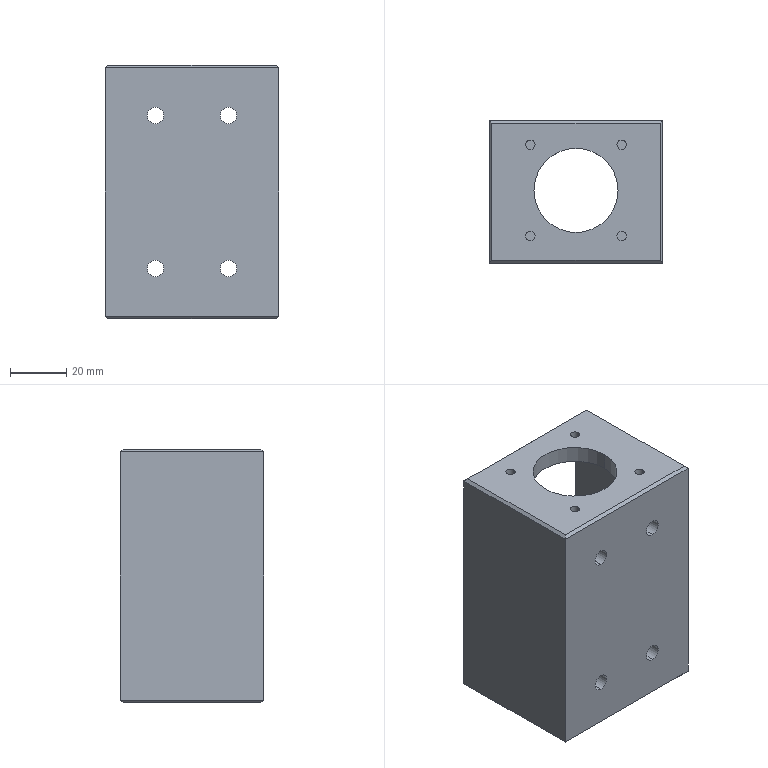Part | Creo | features CURVE 10, CUT 6, DATUM PLANE 3, PROTRUSION 3, CHAMFER 2, COORDINATE SYSTEM 1 | 1 solid | 49 faces | volume 99333 mm3 | cylinder 26 | plane 23 | commonest cylinder face diameters 3.3 x8 5.857 x8 4.2 x6 30 x2 34 x2